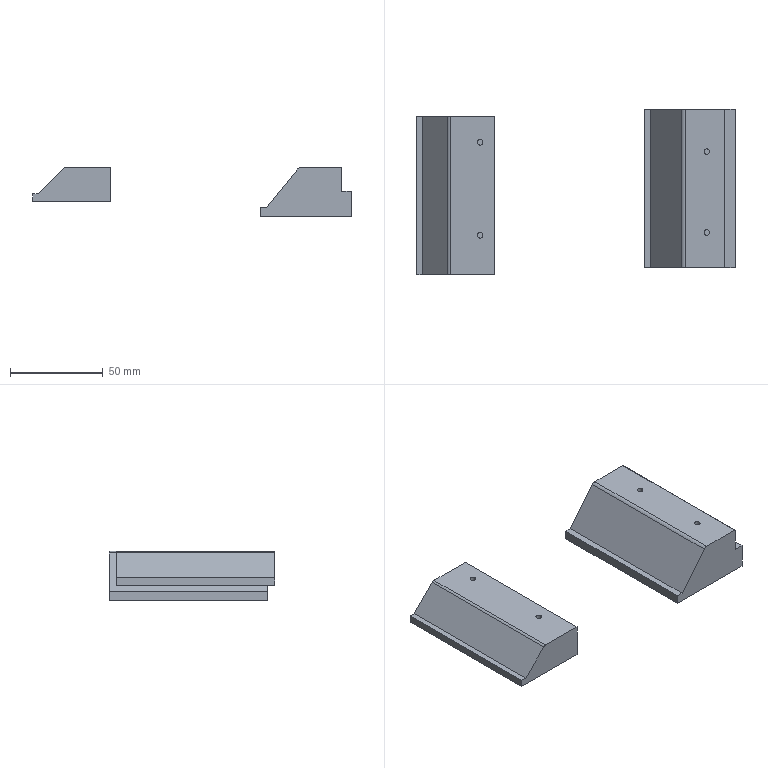NC program | NX | posted with a generic post | part box 171.319 x 88.841 x 26.598 mm
Whole program:
N10 G17 G21 G94 G90
(FLOOR_WALL_COPY_COPY_COPY , TOOL : D80)
N12 T19 M6
N14 G54
N16 G17 G0 G90 X-90.5 Y0. S6500 M3
N18 G43 Z30. H19
N20 Z5.
N22 G94 G1 Z2. F1500.
N24 X-85.5
N26 X85.5
N28 X90.5
N30 Z5.
N32 G0 Z30.
N34 X-90.5
N36 Z4.
N38 G1 Z1.
N40 X-85.5
N42 X85.5
N44 X90.5
N46 Z4.
N48 G0 Z30.
N50 X-90.5
N52 Z3.
N54 G1 Z0.
N56 X-85.5
N58 X85.5
N60 X90.5
N62 Z3.
N64 G0 Z30.
N66 M5
(PLANAR_MILL_COPY_COPY_COPY_COPY_COPY_COPY_1_COPY_1_COPY_COPY , TOOL : D6A45)
N68 T01 M6
N70 G54
N72 G17 G0 G90 X-1.27 Y26.6 S9500 M3
N74 G43 Z30. H1
N76 Z0.5
N78 G94 G1 Z-1. F1250.
N80 X-0.866 Y25.9
N82 G3 X0. Y25.4 R1.
N84 G1 X42.4
N86 G2 X43.4 Y24.4 R1.
N88 G1 Y-24.4
N90 G2 X42.4 Y-25.4 R1.
N92 G1 X-42.4
N94 G2 X-43.4 Y-24.4 R1.
N96 G1 Y24.4
N98 G2 X-42.4 Y25.4 R1.
N100 G1 X0.
N102 G3 X0.866 Y25.9 R1.
N104 G1 X1.27 Y26.6
N106 Z0.5
N108 G0 Z30.
N110 M5
N112 M2